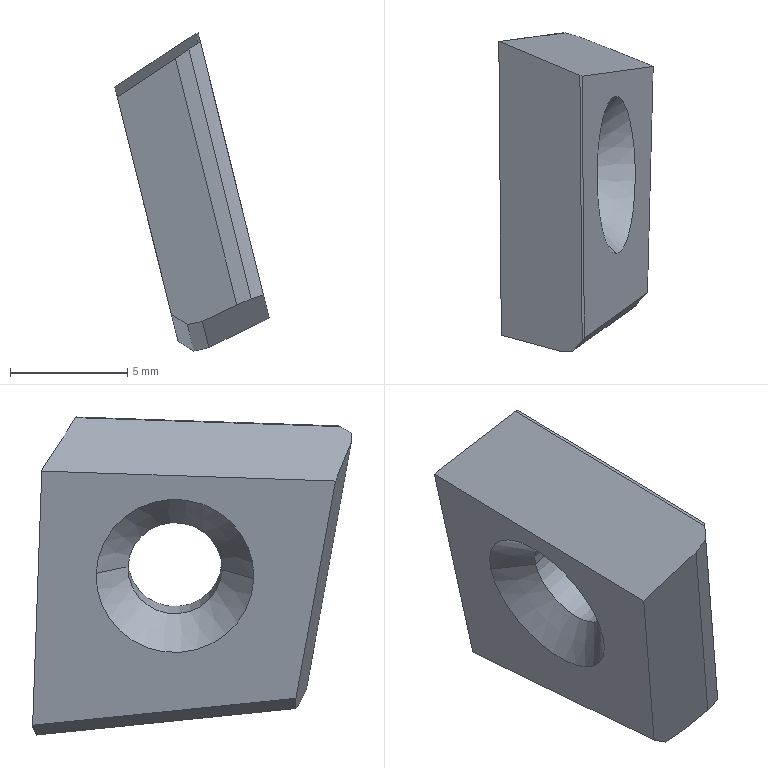Part | SolidWorks | features BaseBody 1 | 1 solid | 18 faces | box 6.573 x 13.574 x 13.543 mm | volume 441.905 mm3 | plane 12 | cone 4 | cylinder 2 | commonest cylinder face diameters 4 x2
STEP:
#1=CARTESIAN_POINT('',(-2059.856,542.741,-1550.749));
#2=VERTEX_POINT('',#1);
#3=CARTESIAN_POINT('',(-2058.548,544.1,-1550.374));
#4=VERTEX_POINT('',#3);
#5=CARTESIAN_POINT('',(-2059.856,542.741,-1550.749));
#6=DIRECTION('',(0.6801,0.7067,0.195));
#7=VECTOR('',#6,1000.);
#8=LINE('',#5,#7);
#9=EDGE_CURVE('',#2,#4,#8,.T.);
#10=ORIENTED_EDGE('',*,*,#9,.T.);
#11=CARTESIAN_POINT('',(-2058.491,537.384,-1550.601));
#12=VERTEX_POINT('',#11);
#13=CARTESIAN_POINT('',(-2058.519,540.742,-1550.487));
#14=DIRECTION('',(0.9703,0.,0.2419));
#15=DIRECTION('',(-0.008443,0.9994,0.03386));
#16=AXIS2_PLACEMENT_3D('',#13,#14,#15);
#17=CIRCLE('',#16,3.36);
#18=EDGE_CURVE('',#4,#12,#17,.T.);
#19=ORIENTED_EDGE('',*,*,#18,.T.);
#20=CARTESIAN_POINT('',(-2059.822,538.743,-1550.884));
#21=VERTEX_POINT('',#20);
#22=CARTESIAN_POINT('',(-2058.491,537.384,-1550.601));
#23=DIRECTION('',(-0.6921,0.7067,-0.1471));
#24=VECTOR('',#23,1000.);
#25=LINE('',#22,#24);
#26=EDGE_CURVE('',#12,#21,#25,.T.);
#27=ORIENTED_EDGE('',*,*,#26,.T.);
#28=CARTESIAN_POINT('',(-2059.839,540.742,-1550.816));
#29=DIRECTION('',(0.9703,0.,0.2419));
#30=DIRECTION('',(-0.008443,0.9994,0.03386));
#31=AXIS2_PLACEMENT_3D('',#28,#29,#30);
#32=CIRCLE('',#31,2.);
#33=EDGE_CURVE('',#2,#21,#32,.T.);
#34=ORIENTED_EDGE('',*,*,#33,.F.);
#35=EDGE_LOOP('',(#10,#19,#27,#34));
#36=FACE_OUTER_BOUND('',#35,.T.);
#37=CARTESIAN_POINT('',(-2059.905,540.742,-1550.833));
#38=DIRECTION('',(0.9703,0.,0.2419));
#39=DIRECTION('',(0.02948,-0.9925,-0.1182));
#40=AXIS2_PLACEMENT_3D('',#37,#38,#39);
#41=CONICAL_SURFACE('',#40,1.932,0.7854);
#42=ADVANCED_FACE('',(#36),#41,.F.);
#43=CARTESIAN_POINT('',(-2061.064,538.743,-1551.194));
#44=VERTEX_POINT('',#43);
#45=CARTESIAN_POINT('',(-2062.372,537.384,-1551.569));
#46=VERTEX_POINT('',#45);
#47=CARTESIAN_POINT('',(-2061.064,538.743,-1551.194));
#48=DIRECTION('',(-0.6801,-0.7067,-0.195));
#49=VECTOR('',#48,1000.);
#50=LINE('',#47,#49);
#51=EDGE_CURVE('',#44,#46,#50,.T.);
#52=ORIENTED_EDGE('',*,*,#51,.T.);
#53=CARTESIAN_POINT('',(-2062.429,544.1,-1551.341));
#54=VERTEX_POINT('',#53);
#55=CARTESIAN_POINT('',(-2062.4,540.742,-1551.455));
#56=DIRECTION('',(-0.9703,0.,-0.2419));
#57=DIRECTION('',(0.008443,-0.9994,-0.03386));
#58=AXIS2_PLACEMENT_3D('',#55,#56,#57);
#59=CIRCLE('',#58,3.36);
#60=EDGE_CURVE('',#46,#54,#59,.T.);
#61=ORIENTED_EDGE('',*,*,#60,.T.);
#62=CARTESIAN_POINT('',(-2061.098,542.741,-1551.058));
#63=VERTEX_POINT('',#62);
#64=CARTESIAN_POINT('',(-2062.429,544.1,-1551.341));
#65=DIRECTION('',(0.6921,-0.7067,0.1471));
#66=VECTOR('',#65,1000.);
#67=LINE('',#64,#66);
#68=EDGE_CURVE('',#54,#63,#67,.T.);
#69=ORIENTED_EDGE('',*,*,#68,.T.);
#70=CARTESIAN_POINT('',(-2061.081,540.742,-1551.126));
#71=DIRECTION('',(-0.9703,0.,-0.2419));
#72=DIRECTION('',(0.008443,-0.9994,-0.03386));
#73=AXIS2_PLACEMENT_3D('',#70,#71,#72);
#74=CIRCLE('',#73,2.);
#75=EDGE_CURVE('',#44,#63,#74,.T.);
#76=ORIENTED_EDGE('',*,*,#75,.F.);
#77=EDGE_LOOP('',(#52,#61,#69,#76));
#78=FACE_OUTER_BOUND('',#77,.T.);
#79=CARTESIAN_POINT('',(-2061.015,540.742,-1551.11));
#80=DIRECTION('',(-0.9703,0.,-0.2419));
#81=DIRECTION('',(0.01266,0.9986,-0.05078));
#82=AXIS2_PLACEMENT_3D('',#79,#80,#81);
#83=CONICAL_SURFACE('',#82,1.932,0.7854);
#84=ADVANCED_FACE('',(#78),#83,.F.);
#85=CARTESIAN_POINT('',(-2061.098,542.741,-1551.058));
#86=DIRECTION('',(0.9703,0.,0.2419));
#87=VECTOR('',#86,1000.);
#88=LINE('',#85,#87);
#89=EDGE_CURVE('',#63,#2,#88,.T.);
#90=ORIENTED_EDGE('',*,*,#89,.T.);
#91=ORIENTED_EDGE('',*,*,#33,.T.);
#92=CARTESIAN_POINT('',(-2059.822,538.743,-1550.884));
#93=DIRECTION('',(-0.9703,0.,-0.2419));
#94=VECTOR('',#93,1000.);
#95=LINE('',#92,#94);
#96=EDGE_CURVE('',#21,#44,#95,.T.);
#97=ORIENTED_EDGE('',*,*,#96,.T.);
#98=ORIENTED_EDGE('',*,*,#75,.T.);
#99=EDGE_LOOP('',(#90,#91,#97,#98));
#100=FACE_OUTER_BOUND('',#99,.T.);
#101=CARTESIAN_POINT('',(-2059.777,540.742,-1550.801));
#102=DIRECTION('',(-0.9703,0.,-0.2419));
#103=DIRECTION('',(0.02948,-0.9925,-0.1182));
#104=AXIS2_PLACEMENT_3D('',#101,#102,#103);
#105=CYLINDRICAL_SURFACE('',#104,2.);
#106=ADVANCED_FACE('',(#100),#105,.F.);
#107=CARTESIAN_POINT('',(-2060.815,546.803,-1557.812));
#108=VERTEX_POINT('',#107);
#109=CARTESIAN_POINT('',(-2060.693,546.798,-1557.89));
#110=VERTEX_POINT('',#109);
#111=CARTESIAN_POINT('',(-2060.815,546.803,-1557.812));
#112=DIRECTION('',(0.8428,-0.03489,-0.5372));
#113=VECTOR('',#112,1000.);
#114=LINE('',#111,#113);
#115=EDGE_CURVE('',#108,#110,#114,.T.);
#116=ORIENTED_EDGE('',*,*,#115,.F.);
#117=CARTESIAN_POINT('',(-2063.513,546.413,-1546.991));
#118=VERTEX_POINT('',#117);
#119=CARTESIAN_POINT('',(-2063.513,546.413,-1546.991));
#120=DIRECTION('',(0.2418,0.0349,-0.9697));
#121=VECTOR('',#120,1000.);
#122=LINE('',#119,#121);
#123=EDGE_CURVE('',#118,#108,#122,.T.);
#124=ORIENTED_EDGE('',*,*,#123,.F.);
#125=CARTESIAN_POINT('',(-2063.425,546.403,-1546.932));
#126=VERTEX_POINT('',#125);
#127=CARTESIAN_POINT('',(-2063.425,546.403,-1546.932));
#128=DIRECTION('',(-0.827,0.09378,-0.5543));
#129=VECTOR('',#128,1000.);
#130=LINE('',#127,#129);
#131=EDGE_CURVE('',#126,#118,#130,.T.);
#132=ORIENTED_EDGE('',*,*,#131,.F.);
#133=CARTESIAN_POINT('',(-2060.693,546.798,-1557.89));
#134=DIRECTION('',(-0.2418,-0.0349,0.9697));
#135=VECTOR('',#134,1000.);
#136=LINE('',#133,#135);
#137=EDGE_CURVE('',#110,#126,#136,.T.);
#138=ORIENTED_EDGE('',*,*,#137,.F.);
#139=EDGE_LOOP('',(#116,#124,#132,#138));
#140=FACE_OUTER_BOUND('',#139,.T.);
#141=CARTESIAN_POINT('',(-2064.205,546.442,-1546.542));
#142=DIRECTION('',(0.07616,0.9956,0.05482));
#143=DIRECTION('',(0.5842,0.,-0.8116));
#144=AXIS2_PLACEMENT_3D('',#141,#142,#143);
#145=PLANE('',#144);
#146=ADVANCED_FACE('',(#140),#145,.T.);
#147=CARTESIAN_POINT('',(-2059.871,533.784,-1545.065));
#148=VERTEX_POINT('',#147);
#149=CARTESIAN_POINT('',(-2059.965,533.679,-1545.101));
#150=VERTEX_POINT('',#149);
#151=CARTESIAN_POINT('',(-2059.871,533.784,-1545.065));
#152=DIRECTION('',(-0.6467,-0.7209,-0.2492));
#153=VECTOR('',#152,1000.);
#154=LINE('',#151,#153);
#155=EDGE_CURVE('',#148,#150,#154,.T.);
#156=ORIENTED_EDGE('',*,*,#155,.F.);
#157=CARTESIAN_POINT('',(-2059.965,544.936,-1544.687));
#158=VERTEX_POINT('',#157);
#159=CARTESIAN_POINT('',(-2059.965,544.936,-1544.687));
#160=DIRECTION('',(0.008443,-0.9994,-0.03386));
#161=VECTOR('',#160,1000.);
#162=LINE('',#159,#161);
#163=EDGE_CURVE('',#158,#148,#162,.T.);
#164=ORIENTED_EDGE('',*,*,#163,.F.);
#165=CARTESIAN_POINT('',(-2060.061,544.973,-1544.718));
#166=VERTEX_POINT('',#165);
#167=CARTESIAN_POINT('',(-2060.061,544.973,-1544.718));
#168=DIRECTION('',(0.8918,-0.3435,0.2945));
#169=VECTOR('',#168,1000.);
#170=LINE('',#167,#169);
#171=EDGE_CURVE('',#166,#158,#170,.T.);
#172=ORIENTED_EDGE('',*,*,#171,.F.);
#173=CARTESIAN_POINT('',(-2059.965,533.679,-1545.101));
#174=DIRECTION('',(-0.008443,0.9994,0.03386));
#175=VECTOR('',#174,1000.);
#176=LINE('',#173,#175);
#177=EDGE_CURVE('',#150,#166,#176,.T.);
#178=ORIENTED_EDGE('',*,*,#177,.F.);
#179=EDGE_LOOP('',(#156,#164,#172,#178));
#180=FACE_OUTER_BOUND('',#179,.T.);
#181=CARTESIAN_POINT('',(-2060.495,533.116,-1545.304));
#182=DIRECTION('',(-0.3254,-0.03477,0.9449));
#183=DIRECTION('',(-0.1062,0.9943,0.));
#184=AXIS2_PLACEMENT_3D('',#181,#182,#183);
#185=PLANE('',#184);
#186=ADVANCED_FACE('',(#180),#185,.T.);
#187=CARTESIAN_POINT('',(-2061.101,535.591,-1556.669));
#188=VERTEX_POINT('',#187);
#189=CARTESIAN_POINT('',(-2060.815,546.803,-1557.812));
#190=DIRECTION('',(-0.02529,-0.9945,0.1014));
#191=VECTOR('',#190,1000.);
#192=LINE('',#189,#191);
#193=EDGE_CURVE('',#108,#188,#192,.T.);
#194=ORIENTED_EDGE('',*,*,#193,.F.);
#195=ORIENTED_EDGE('',*,*,#115,.T.);
#196=CARTESIAN_POINT('',(-2060.144,546.65,-1558.229));
#197=VERTEX_POINT('',#196);
#198=CARTESIAN_POINT('',(-2060.144,546.65,-1558.229));
#199=DIRECTION('',(-0.8292,0.2235,0.5123));
#200=VECTOR('',#199,1000.);
#201=LINE('',#198,#200);
#202=EDGE_CURVE('',#197,#110,#201,.T.);
#203=ORIENTED_EDGE('',*,*,#202,.F.);
#204=CARTESIAN_POINT('',(-2060.425,535.596,-1557.102));
#205=VERTEX_POINT('',#204);
#206=CARTESIAN_POINT('',(-2060.425,535.596,-1557.102));
#207=DIRECTION('',(0.02529,0.9945,-0.1014));
#208=VECTOR('',#207,1000.);
#209=LINE('',#206,#208);
#210=EDGE_CURVE('',#205,#197,#209,.T.);
#211=ORIENTED_EDGE('',*,*,#210,.F.);
#212=CARTESIAN_POINT('',(-2061.101,535.591,-1556.669));
#213=DIRECTION('',(0.8417,0.005443,-0.5399));
#214=VECTOR('',#213,1000.);
#215=LINE('',#212,#214);
#216=EDGE_CURVE('',#188,#205,#215,.T.);
#217=ORIENTED_EDGE('',*,*,#216,.F.);
#218=EDGE_LOOP('',(#194,#195,#203,#211,#217));
#219=FACE_OUTER_BOUND('',#218,.T.);
#220=CARTESIAN_POINT('',(-2058.972,535.079,-1557.989));
#221=DIRECTION('',(-0.5382,-0.07195,-0.8397));
#222=DIRECTION('',(-0.8419,0.,0.5396));
#223=AXIS2_PLACEMENT_3D('',#220,#221,#222);
#224=PLANE('',#223);
#225=ADVANCED_FACE('',(#219),#224,.T.);
#226=CARTESIAN_POINT('',(-2057.185,535.741,-1555.837));
#227=VERTEX_POINT('',#226);
#228=CARTESIAN_POINT('',(-2059.871,533.784,-1545.065));
#229=DIRECTION('',(0.2382,0.1736,-0.9556));
#230=VECTOR('',#229,1000.);
#231=LINE('',#228,#230);
#232=EDGE_CURVE('',#148,#227,#231,.T.);
#233=ORIENTED_EDGE('',*,*,#232,.F.);
#234=ORIENTED_EDGE('',*,*,#155,.T.);
#235=CARTESIAN_POINT('',(-2060.359,533.229,-1545.384));
#236=VERTEX_POINT('',#235);
#237=CARTESIAN_POINT('',(-2060.359,533.229,-1545.384));
#238=DIRECTION('',(0.5947,0.6804,0.4282));
#239=VECTOR('',#238,1000.);
#240=LINE('',#237,#239);
#241=EDGE_CURVE('',#236,#150,#240,.T.);
#242=ORIENTED_EDGE('',*,*,#241,.F.);
#243=CARTESIAN_POINT('',(-2057.711,535.159,-1556.005));
#244=VERTEX_POINT('',#243);
#245=CARTESIAN_POINT('',(-2057.711,535.159,-1556.005));
#246=DIRECTION('',(-0.2382,-0.1736,0.9556));
#247=VECTOR('',#246,1000.);
#248=LINE('',#245,#247);
#249=EDGE_CURVE('',#244,#236,#248,.T.);
#250=ORIENTED_EDGE('',*,*,#249,.F.);
#251=CARTESIAN_POINT('',(-2057.185,535.741,-1555.837));
#252=DIRECTION('',(-0.6547,-0.7261,-0.2099));
#253=VECTOR('',#252,1000.);
#254=LINE('',#251,#253);
#255=EDGE_CURVE('',#227,#244,#254,.T.);
#256=ORIENTED_EDGE('',*,*,#255,.F.);
#257=EDGE_LOOP('',(#233,#234,#242,#250,#256));
#258=FACE_OUTER_BOUND('',#257,.T.);
#259=CARTESIAN_POINT('',(-2058.846,534.969,-1544.19));
#260=DIRECTION('',(0.7327,-0.6779,0.0595));
#261=DIRECTION('',(0.,-0.08744,-0.9962));
#262=AXIS2_PLACEMENT_3D('',#259,#260,#261);
#263=PLANE('',#262);
#264=ADVANCED_FACE('',(#258),#263,.T.);
#265=CARTESIAN_POINT('',(-2059.784,535.483,-1556.967));
#266=VERTEX_POINT('',#265);
#267=CARTESIAN_POINT('',(-2060.425,535.596,-1557.102));
#268=DIRECTION('',(0.9645,-0.1698,0.2024));
#269=VECTOR('',#268,1000.);
#270=LINE('',#267,#269);
#271=EDGE_CURVE('',#205,#266,#270,.T.);
#272=ORIENTED_EDGE('',*,*,#271,.F.);
#273=ORIENTED_EDGE('',*,*,#210,.T.);
#274=CARTESIAN_POINT('',(-2059.506,546.412,-1558.082));
#275=VERTEX_POINT('',#274);
#276=CARTESIAN_POINT('',(-2059.506,546.412,-1558.082));
#277=DIRECTION('',(-0.9157,0.3417,-0.2115));
#278=VECTOR('',#277,1000.);
#279=LINE('',#276,#278);
#280=EDGE_CURVE('',#275,#197,#279,.T.);
#281=ORIENTED_EDGE('',*,*,#280,.F.);
#282=CARTESIAN_POINT('',(-2059.784,535.483,-1556.967));
#283=DIRECTION('',(0.02529,0.9945,-0.1014));
#284=VECTOR('',#283,1000.);
#285=LINE('',#282,#284);
#286=EDGE_CURVE('',#266,#275,#285,.T.);
#287=ORIENTED_EDGE('',*,*,#286,.F.);
#288=EDGE_LOOP('',(#272,#273,#281,#287));
#289=FACE_OUTER_BOUND('',#288,.T.);
#290=CARTESIAN_POINT('',(-2060.993,534.932,-1557.139));
#291=DIRECTION('',(0.1866,-0.1044,-0.9769));
#292=DIRECTION('',(0.,-0.9943,0.1062));
#293=AXIS2_PLACEMENT_3D('',#290,#291,#292);
#294=PLANE('',#293);
#295=ADVANCED_FACE('',(#289),#294,.T.);
#296=CARTESIAN_POINT('',(-2058.319,535.142,-1556.275));
#297=VERTEX_POINT('',#296);
#298=CARTESIAN_POINT('',(-2057.711,535.159,-1556.005));
#299=DIRECTION('',(-0.9139,-0.025,-0.4051));
#300=VECTOR('',#299,1000.);
#301=LINE('',#298,#300);
#302=EDGE_CURVE('',#244,#297,#301,.T.);
#303=ORIENTED_EDGE('',*,*,#302,.F.);
#304=ORIENTED_EDGE('',*,*,#249,.T.);
#305=CARTESIAN_POINT('',(-2060.937,533.234,-1545.774));
#306=VERTEX_POINT('',#305);
#307=CARTESIAN_POINT('',(-2060.937,533.234,-1545.774));
#308=DIRECTION('',(0.829,-0.007507,0.5591));
#309=VECTOR('',#308,1000.);
#310=LINE('',#307,#309);
#311=EDGE_CURVE('',#306,#236,#310,.T.);
#312=ORIENTED_EDGE('',*,*,#311,.F.);
#313=CARTESIAN_POINT('',(-2058.319,535.142,-1556.275));
#314=DIRECTION('',(-0.2382,-0.1736,0.9556));
#315=VECTOR('',#314,1000.);
#316=LINE('',#313,#315);
#317=EDGE_CURVE('',#297,#306,#316,.T.);
#318=ORIENTED_EDGE('',*,*,#317,.F.);
#319=EDGE_LOOP('',(#303,#304,#312,#318));
#320=FACE_OUTER_BOUND('',#319,.T.);
#321=CARTESIAN_POINT('',(-2057.008,535.306,-1556.506));
#322=DIRECTION('',(0.09554,-0.9833,-0.1549));
#323=DIRECTION('',(0.,0.1556,-0.9878));
#324=AXIS2_PLACEMENT_3D('',#321,#322,#323);
#325=PLANE('',#324);
#326=ADVANCED_FACE('',(#320),#325,.T.);
#327=CARTESIAN_POINT('',(-2056.941,545.373,-1556.819));
#328=VERTEX_POINT('',#327);
#329=CARTESIAN_POINT('',(-2056.941,545.373,-1556.819));
#330=DIRECTION('',(-0.02529,-0.9945,0.1014));
#331=VECTOR('',#330,1000.);
#332=LINE('',#329,#331);
#333=EDGE_CURVE('',#328,#227,#332,.T.);
#334=ORIENTED_EDGE('',*,*,#333,.T.);
#335=ORIENTED_EDGE('',*,*,#255,.T.);
#336=ORIENTED_EDGE('',*,*,#302,.T.);
#337=CARTESIAN_POINT('',(-2059.784,535.483,-1556.967));
#338=DIRECTION('',(0.8848,-0.2056,0.4182));
#339=VECTOR('',#338,1000.);
#340=LINE('',#337,#339);
#341=EDGE_CURVE('',#266,#297,#340,.T.);
#342=ORIENTED_EDGE('',*,*,#341,.F.);
#343=ORIENTED_EDGE('',*,*,#286,.T.);
#344=CARTESIAN_POINT('',(-2059.506,546.412,-1558.082));
#345=DIRECTION('',(0.8433,-0.3415,0.4151));
#346=VECTOR('',#345,1000.);
#347=LINE('',#344,#346);
#348=EDGE_CURVE('',#275,#328,#347,.T.);
#349=ORIENTED_EDGE('',*,*,#348,.T.);
#350=EDGE_LOOP('',(#334,#335,#336,#342,#343,#349));
#351=FACE_OUTER_BOUND('',#350,.T.);
#352=CARTESIAN_POINT('',(-2056.725,534.568,-1555.498));
#353=DIRECTION('',(0.4054,-0.1029,-0.9083));
#354=DIRECTION('',(0.,-0.9936,0.1126));
#355=AXIS2_PLACEMENT_3D('',#352,#353,#354);
#356=PLANE('',#355);
#357=ADVANCED_FACE('',(#351),#356,.T.);
#358=ORIENTED_EDGE('',*,*,#26,.F.);
#359=CARTESIAN_POINT('',(-2058.519,540.742,-1550.487));
#360=DIRECTION('',(0.9703,0.,0.2419));
#361=DIRECTION('',(0.008443,-0.9994,-0.03386));
#362=AXIS2_PLACEMENT_3D('',#359,#360,#361);
#363=CIRCLE('',#362,3.36);
#364=EDGE_CURVE('',#12,#4,#363,.T.);
#365=ORIENTED_EDGE('',*,*,#364,.T.);
#366=ORIENTED_EDGE('',*,*,#9,.F.);
#367=CARTESIAN_POINT('',(-2059.839,540.742,-1550.816));
#368=DIRECTION('',(0.9703,0.,0.2419));
#369=DIRECTION('',(0.008443,-0.9994,-0.03386));
#370=AXIS2_PLACEMENT_3D('',#367,#368,#369);
#371=CIRCLE('',#370,2.);
#372=EDGE_CURVE('',#21,#2,#371,.T.);
#373=ORIENTED_EDGE('',*,*,#372,.F.);
#374=EDGE_LOOP('',(#358,#365,#366,#373));
#375=FACE_OUTER_BOUND('',#374,.T.);
#376=CARTESIAN_POINT('',(-2059.905,540.742,-1550.833));
#377=DIRECTION('',(0.9703,0.,0.2419));
#378=DIRECTION('',(-0.02948,0.9925,0.1182));
#379=AXIS2_PLACEMENT_3D('',#376,#377,#378);
#380=CONICAL_SURFACE('',#379,1.932,0.7854);
#381=ADVANCED_FACE('',(#375),#380,.F.);
#382=ORIENTED_EDGE('',*,*,#68,.F.);
#383=CARTESIAN_POINT('',(-2062.4,540.742,-1551.455));
#384=DIRECTION('',(-0.9703,0.,-0.2419));
#385=DIRECTION('',(-0.008443,0.9994,0.03386));
#386=AXIS2_PLACEMENT_3D('',#383,#384,#385);
#387=CIRCLE('',#386,3.36);
#388=EDGE_CURVE('',#54,#46,#387,.T.);
#389=ORIENTED_EDGE('',*,*,#388,.T.);
#390=ORIENTED_EDGE('',*,*,#51,.F.);
#391=CARTESIAN_POINT('',(-2061.081,540.742,-1551.126));
#392=DIRECTION('',(-0.9703,0.,-0.2419));
#393=DIRECTION('',(-0.008443,0.9994,0.03386));
#394=AXIS2_PLACEMENT_3D('',#391,#392,#393);
#395=CIRCLE('',#394,2.);
#396=EDGE_CURVE('',#63,#44,#395,.T.);
#397=ORIENTED_EDGE('',*,*,#396,.F.);
#398=EDGE_LOOP('',(#382,#389,#390,#397));
#399=FACE_OUTER_BOUND('',#398,.T.);
#400=CARTESIAN_POINT('',(-2061.015,540.742,-1551.11));
#401=DIRECTION('',(-0.9703,0.,-0.2419));
#402=DIRECTION('',(-0.01266,-0.9986,0.05078));
#403=AXIS2_PLACEMENT_3D('',#400,#401,#402);
#404=CONICAL_SURFACE('',#403,1.932,0.7854);
#405=ADVANCED_FACE('',(#399),#404,.F.);
#406=ORIENTED_EDGE('',*,*,#96,.F.);
#407=ORIENTED_EDGE('',*,*,#372,.T.);
#408=ORIENTED_EDGE('',*,*,#89,.F.);
#409=ORIENTED_EDGE('',*,*,#396,.T.);
#410=EDGE_LOOP('',(#406,#407,#408,#409));
#411=FACE_OUTER_BOUND('',#410,.T.);
#412=CARTESIAN_POINT('',(-2059.777,540.742,-1550.801));
#413=DIRECTION('',(-0.9703,0.,-0.2419));
#414=DIRECTION('',(-0.02948,0.9925,0.1182));
#415=AXIS2_PLACEMENT_3D('',#412,#413,#414);
#416=CYLINDRICAL_SURFACE('',#415,2.);
#417=ADVANCED_FACE('',(#411),#416,.F.);
#418=CARTESIAN_POINT('',(-2063.425,546.403,-1546.932));
#419=DIRECTION('',(0.7872,-0.3347,0.518));
#420=VECTOR('',#419,1000.);
#421=LINE('',#418,#420);
#422=EDGE_CURVE('',#126,#166,#421,.T.);
#423=ORIENTED_EDGE('',*,*,#422,.F.);
#424=ORIENTED_EDGE('',*,*,#131,.T.);
#425=CARTESIAN_POINT('',(-2063.408,533.91,-1547.415));
#426=VERTEX_POINT('',#425);
#427=CARTESIAN_POINT('',(-2063.408,533.91,-1547.415));
#428=DIRECTION('',(-0.008443,0.9994,0.03386));
#429=VECTOR('',#428,1000.);
#430=LINE('',#427,#429);
#431=EDGE_CURVE('',#426,#118,#430,.T.);
#432=ORIENTED_EDGE('',*,*,#431,.F.);
#433=CARTESIAN_POINT('',(-2063.408,533.91,-1547.415));
#434=DIRECTION('',(0.8123,-0.2221,0.5393));
#435=VECTOR('',#434,1000.);
#436=LINE('',#433,#435);
#437=EDGE_CURVE('',#426,#306,#436,.T.);
#438=ORIENTED_EDGE('',*,*,#437,.T.);
#439=ORIENTED_EDGE('',*,*,#311,.T.);
#440=ORIENTED_EDGE('',*,*,#241,.T.);
#441=ORIENTED_EDGE('',*,*,#177,.T.);
#442=EDGE_LOOP('',(#423,#424,#432,#438,#439,#440,#441));
#443=FACE_OUTER_BOUND('',#442,.T.);
#444=CARTESIAN_POINT('',(-2063.942,532.62,-1547.826));
#445=DIRECTION('',(-0.5591,-0.03279,0.8285));
#446=DIRECTION('',(-0.05856,0.9983,0.));
#447=AXIS2_PLACEMENT_3D('',#444,#445,#446);
#448=PLANE('',#447);
#449=ADVANCED_FACE('',(#443),#448,.T.);
#450=ORIENTED_EDGE('',*,*,#202,.T.);
#451=ORIENTED_EDGE('',*,*,#137,.T.);
#452=ORIENTED_EDGE('',*,*,#422,.T.);
#453=ORIENTED_EDGE('',*,*,#171,.T.);
#454=CARTESIAN_POINT('',(-2056.941,545.373,-1556.819));
#455=DIRECTION('',(-0.2418,-0.0349,0.9697));
#456=VECTOR('',#455,1000.);
#457=LINE('',#454,#456);
#458=EDGE_CURVE('',#328,#158,#457,.T.);
#459=ORIENTED_EDGE('',*,*,#458,.F.);
#460=ORIENTED_EDGE('',*,*,#348,.F.);
#461=ORIENTED_EDGE('',*,*,#280,.T.);
#462=EDGE_LOOP('',(#450,#451,#452,#453,#459,#460,#461));
#463=FACE_OUTER_BOUND('',#462,.T.);
#464=CARTESIAN_POINT('',(-2056.025,545.193,-1557.936));
#465=DIRECTION('',(0.3239,0.9391,0.1146));
#466=DIRECTION('',(0.3334,0.,-0.9428));
#467=AXIS2_PLACEMENT_3D('',#464,#465,#466);
#468=PLANE('',#467);
#469=ADVANCED_FACE('',(#463),#468,.T.);
#470=ORIENTED_EDGE('',*,*,#18,.F.);
#471=ORIENTED_EDGE('',*,*,#364,.F.);
#472=EDGE_LOOP('',(#470,#471));
#473=FACE_BOUND('',#472,.T.);
#474=ORIENTED_EDGE('',*,*,#458,.T.);
#475=ORIENTED_EDGE('',*,*,#163,.T.);
#476=ORIENTED_EDGE('',*,*,#232,.T.);
#477=ORIENTED_EDGE('',*,*,#333,.F.);
#478=EDGE_LOOP('',(#474,#475,#476,#477));
#479=FACE_OUTER_BOUND('',#478,.T.);
#480=CARTESIAN_POINT('',(-2056.69,533.617,-1557.825));
#481=DIRECTION('',(0.9703,0.,0.2419));
#482=DIRECTION('',(0.,-1.,0.));
#483=AXIS2_PLACEMENT_3D('',#480,#481,#482);
#484=PLANE('',#483);
#485=ADVANCED_FACE('',(#473,#479),#484,.T.);
#486=ORIENTED_EDGE('',*,*,#60,.F.);
#487=ORIENTED_EDGE('',*,*,#388,.F.);
#488=EDGE_LOOP('',(#486,#487));
#489=FACE_BOUND('',#488,.T.);
#490=ORIENTED_EDGE('',*,*,#431,.T.);
#491=ORIENTED_EDGE('',*,*,#123,.T.);
#492=ORIENTED_EDGE('',*,*,#193,.T.);
#493=CARTESIAN_POINT('',(-2061.101,535.591,-1556.669));
#494=DIRECTION('',(-0.2382,-0.1736,0.9556));
#495=VECTOR('',#494,1000.);
#496=LINE('',#493,#495);
#497=EDGE_CURVE('',#188,#426,#496,.T.);
#498=ORIENTED_EDGE('',*,*,#497,.T.);
#499=EDGE_LOOP('',(#490,#491,#492,#498));
#500=FACE_OUTER_BOUND('',#499,.T.);
#501=CARTESIAN_POINT('',(-2063.554,533.263,-1546.829));
#502=DIRECTION('',(-0.9703,0.,-0.2419));
#503=DIRECTION('',(-0.2419,0.,0.9703));
#504=AXIS2_PLACEMENT_3D('',#501,#502,#503);
#505=PLANE('',#504);
#506=ADVANCED_FACE('',(#489,#500),#505,.T.);
#507=ORIENTED_EDGE('',*,*,#497,.F.);
#508=ORIENTED_EDGE('',*,*,#216,.T.);
#509=ORIENTED_EDGE('',*,*,#271,.T.);
#510=ORIENTED_EDGE('',*,*,#341,.T.);
#511=ORIENTED_EDGE('',*,*,#317,.T.);
#512=ORIENTED_EDGE('',*,*,#437,.F.);
#513=EDGE_LOOP('',(#507,#508,#509,#510,#511,#512));
#514=FACE_OUTER_BOUND('',#513,.T.);
#515=CARTESIAN_POINT('',(-2060.543,533.039,-1545.105));
#516=DIRECTION('',(-0.1271,-0.9698,-0.2079));
#517=DIRECTION('',(0.,0.2096,-0.9778));
#518=AXIS2_PLACEMENT_3D('',#515,#516,#517);
#519=PLANE('',#518);
#520=ADVANCED_FACE('',(#514),#519,.T.);
#521=CLOSED_SHELL('',(#42,#84,#106,#146,#186,#225,#264,#295,#326,#357,#381,#405,#417,#449,#469,#485,#506,#520));
#522=MANIFOLD_SOLID_BREP('',#521);
#523=CARTESIAN_POINT('',(0.,0.,0.));
#524=DIRECTION('',(0.,0.,1.));
#525=DIRECTION('',(1.,0.,0.));
#526=AXIS2_PLACEMENT_3D('',#523,#524,#525);
#527=(LENGTH_UNIT()NAMED_UNIT(*)SI_UNIT(.MILLI.,.METRE.));
#528=UNCERTAINTY_MEASURE_WITH_UNIT(LENGTH_MEASURE(0.00001),#527,'','');
#529=(NAMED_UNIT(*)PLANE_ANGLE_UNIT()SI_UNIT($,.RADIAN.));
#530=(NAMED_UNIT(*)SI_UNIT($,.STERADIAN.)SOLID_ANGLE_UNIT());
#531=(GEOMETRIC_REPRESENTATION_CONTEXT(3)GLOBAL_UNCERTAINTY_ASSIGNED_CONTEXT((#528))GLOBAL_UNIT_ASSIGNED_CONTEXT((#527,#529,#530))REPRESENTATION_CONTEXT('',''));
#532=ADVANCED_BREP_SHAPE_REPRESENTATION('',(#522,#526),#531);